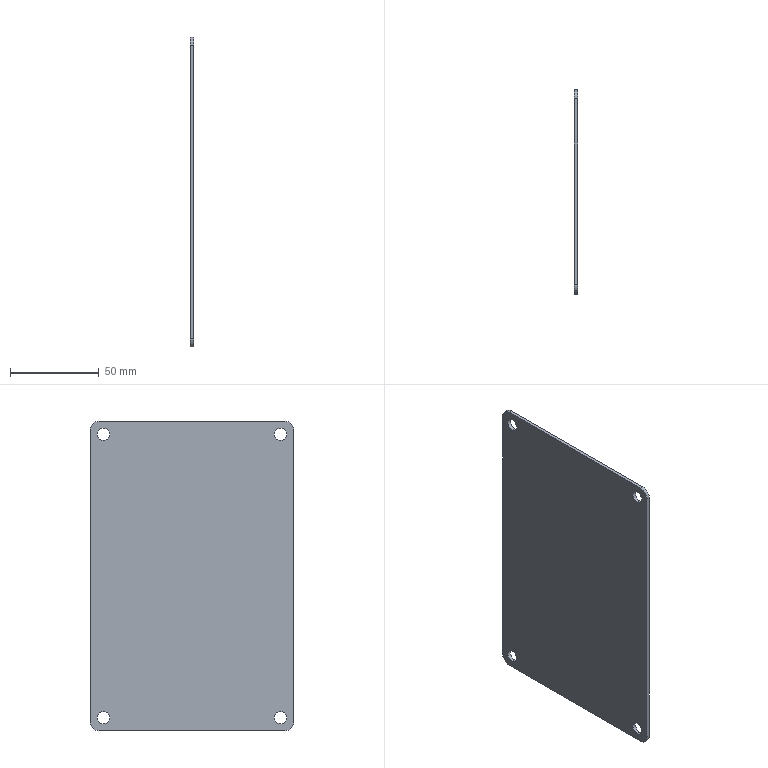Part | SolidWorks | 1 solid | 18 faces | box 2 x 115 x 175 mm | volume 39899 mm3 | cylinder 12 | plane 6 | commonest cylinder face diameters 7 x8 10 x4
STEP:
#1=CARTESIAN_POINT('',(-2.,-50.,76.5));
#2=VERTEX_POINT('',#1);
#3=CARTESIAN_POINT('',(-2.,-50.,83.5));
#4=VERTEX_POINT('',#3);
#5=CARTESIAN_POINT('',(-2.,-50.,80.));
#6=DIRECTION('',(-1.,0.,0.));
#7=DIRECTION('',(0.,0.,-1.));
#8=AXIS2_PLACEMENT_3D('',#5,#6,#7);
#9=CIRCLE('',#8,3.5);
#10=EDGE_CURVE('',#2,#4,#9,.T.);
#11=ORIENTED_EDGE('',*,*,#10,.T.);
#12=CARTESIAN_POINT('',(0.,-50.,83.5));
#13=VERTEX_POINT('',#12);
#14=CARTESIAN_POINT('',(-2.001,-50.,83.5));
#15=DIRECTION('',(1.,0.,0.));
#16=VECTOR('',#15,1000.);
#17=LINE('',#14,#16);
#18=EDGE_CURVE('',#4,#13,#17,.T.);
#19=ORIENTED_EDGE('',*,*,#18,.T.);
#20=CARTESIAN_POINT('',(0.,-50.,76.5));
#21=VERTEX_POINT('',#20);
#22=CARTESIAN_POINT('',(0.,-50.,80.));
#23=DIRECTION('',(1.,0.,0.));
#24=DIRECTION('',(0.,0.,-1.));
#25=AXIS2_PLACEMENT_3D('',#22,#23,#24);
#26=CIRCLE('',#25,3.5);
#27=EDGE_CURVE('',#13,#21,#26,.T.);
#28=ORIENTED_EDGE('',*,*,#27,.T.);
#29=CARTESIAN_POINT('',(-2.001,-50.,76.5));
#30=DIRECTION('',(1.,0.,0.));
#31=VECTOR('',#30,1000.);
#32=LINE('',#29,#31);
#33=EDGE_CURVE('',#2,#21,#32,.T.);
#34=ORIENTED_EDGE('',*,*,#33,.F.);
#35=EDGE_LOOP('',(#11,#19,#28,#34));
#36=FACE_OUTER_BOUND('',#35,.T.);
#37=CARTESIAN_POINT('',(-2.001,-50.,80.));
#38=DIRECTION('',(1.,0.,0.));
#39=DIRECTION('',(0.,0.,-1.));
#40=AXIS2_PLACEMENT_3D('',#37,#38,#39);
#41=CYLINDRICAL_SURFACE('',#40,3.5);
#42=ADVANCED_FACE('',(#36),#41,.F.);
#43=CARTESIAN_POINT('',(-2.,-50.,-83.5));
#44=VERTEX_POINT('',#43);
#45=CARTESIAN_POINT('',(-2.,-50.,-76.5));
#46=VERTEX_POINT('',#45);
#47=CARTESIAN_POINT('',(-2.,-50.,-80.));
#48=DIRECTION('',(-1.,0.,0.));
#49=DIRECTION('',(0.,0.,-1.));
#50=AXIS2_PLACEMENT_3D('',#47,#48,#49);
#51=CIRCLE('',#50,3.5);
#52=EDGE_CURVE('',#44,#46,#51,.T.);
#53=ORIENTED_EDGE('',*,*,#52,.T.);
#54=CARTESIAN_POINT('',(0.,-50.,-76.5));
#55=VERTEX_POINT('',#54);
#56=CARTESIAN_POINT('',(-2.001,-50.,-76.5));
#57=DIRECTION('',(1.,0.,0.));
#58=VECTOR('',#57,1000.);
#59=LINE('',#56,#58);
#60=EDGE_CURVE('',#46,#55,#59,.T.);
#61=ORIENTED_EDGE('',*,*,#60,.T.);
#62=CARTESIAN_POINT('',(0.,-50.,-83.5));
#63=VERTEX_POINT('',#62);
#64=CARTESIAN_POINT('',(0.,-50.,-80.));
#65=DIRECTION('',(1.,0.,0.));
#66=DIRECTION('',(0.,0.,-1.));
#67=AXIS2_PLACEMENT_3D('',#64,#65,#66);
#68=CIRCLE('',#67,3.5);
#69=EDGE_CURVE('',#55,#63,#68,.T.);
#70=ORIENTED_EDGE('',*,*,#69,.T.);
#71=CARTESIAN_POINT('',(-2.001,-50.,-83.5));
#72=DIRECTION('',(1.,0.,0.));
#73=VECTOR('',#72,1000.);
#74=LINE('',#71,#73);
#75=EDGE_CURVE('',#44,#63,#74,.T.);
#76=ORIENTED_EDGE('',*,*,#75,.F.);
#77=EDGE_LOOP('',(#53,#61,#70,#76));
#78=FACE_OUTER_BOUND('',#77,.T.);
#79=CARTESIAN_POINT('',(-2.001,-50.,-80.));
#80=DIRECTION('',(1.,0.,0.));
#81=DIRECTION('',(0.,0.,-1.));
#82=AXIS2_PLACEMENT_3D('',#79,#80,#81);
#83=CYLINDRICAL_SURFACE('',#82,3.5);
#84=ADVANCED_FACE('',(#78),#83,.F.);
#85=CARTESIAN_POINT('',(-2.,50.,-83.5));
#86=VERTEX_POINT('',#85);
#87=CARTESIAN_POINT('',(-2.,50.,-76.5));
#88=VERTEX_POINT('',#87);
#89=CARTESIAN_POINT('',(-2.,50.,-80.));
#90=DIRECTION('',(-1.,0.,0.));
#91=DIRECTION('',(0.,0.,-1.));
#92=AXIS2_PLACEMENT_3D('',#89,#90,#91);
#93=CIRCLE('',#92,3.5);
#94=EDGE_CURVE('',#86,#88,#93,.T.);
#95=ORIENTED_EDGE('',*,*,#94,.T.);
#96=CARTESIAN_POINT('',(0.,50.,-76.5));
#97=VERTEX_POINT('',#96);
#98=CARTESIAN_POINT('',(-2.001,50.,-76.5));
#99=DIRECTION('',(1.,0.,0.));
#100=VECTOR('',#99,1000.);
#101=LINE('',#98,#100);
#102=EDGE_CURVE('',#88,#97,#101,.T.);
#103=ORIENTED_EDGE('',*,*,#102,.T.);
#104=CARTESIAN_POINT('',(0.,50.,-83.5));
#105=VERTEX_POINT('',#104);
#106=CARTESIAN_POINT('',(0.,50.,-80.));
#107=DIRECTION('',(1.,0.,0.));
#108=DIRECTION('',(0.,0.,-1.));
#109=AXIS2_PLACEMENT_3D('',#106,#107,#108);
#110=CIRCLE('',#109,3.5);
#111=EDGE_CURVE('',#97,#105,#110,.T.);
#112=ORIENTED_EDGE('',*,*,#111,.T.);
#113=CARTESIAN_POINT('',(-2.001,50.,-83.5));
#114=DIRECTION('',(1.,0.,0.));
#115=VECTOR('',#114,1000.);
#116=LINE('',#113,#115);
#117=EDGE_CURVE('',#86,#105,#116,.T.);
#118=ORIENTED_EDGE('',*,*,#117,.F.);
#119=EDGE_LOOP('',(#95,#103,#112,#118));
#120=FACE_OUTER_BOUND('',#119,.T.);
#121=CARTESIAN_POINT('',(-2.001,50.,-80.));
#122=DIRECTION('',(1.,0.,0.));
#123=DIRECTION('',(0.,0.,-1.));
#124=AXIS2_PLACEMENT_3D('',#121,#122,#123);
#125=CYLINDRICAL_SURFACE('',#124,3.5);
#126=ADVANCED_FACE('',(#120),#125,.F.);
#127=CARTESIAN_POINT('',(-2.,50.,76.5));
#128=VERTEX_POINT('',#127);
#129=CARTESIAN_POINT('',(-2.,50.,83.5));
#130=VERTEX_POINT('',#129);
#131=CARTESIAN_POINT('',(-2.,50.,80.));
#132=DIRECTION('',(-1.,0.,0.));
#133=DIRECTION('',(0.,0.,-1.));
#134=AXIS2_PLACEMENT_3D('',#131,#132,#133);
#135=CIRCLE('',#134,3.5);
#136=EDGE_CURVE('',#128,#130,#135,.T.);
#137=ORIENTED_EDGE('',*,*,#136,.T.);
#138=CARTESIAN_POINT('',(0.,50.,83.5));
#139=VERTEX_POINT('',#138);
#140=CARTESIAN_POINT('',(-2.001,50.,83.5));
#141=DIRECTION('',(1.,0.,0.));
#142=VECTOR('',#141,1000.);
#143=LINE('',#140,#142);
#144=EDGE_CURVE('',#130,#139,#143,.T.);
#145=ORIENTED_EDGE('',*,*,#144,.T.);
#146=CARTESIAN_POINT('',(0.,50.,76.5));
#147=VERTEX_POINT('',#146);
#148=CARTESIAN_POINT('',(0.,50.,80.));
#149=DIRECTION('',(1.,0.,0.));
#150=DIRECTION('',(0.,0.,-1.));
#151=AXIS2_PLACEMENT_3D('',#148,#149,#150);
#152=CIRCLE('',#151,3.5);
#153=EDGE_CURVE('',#139,#147,#152,.T.);
#154=ORIENTED_EDGE('',*,*,#153,.T.);
#155=CARTESIAN_POINT('',(-2.001,50.,76.5));
#156=DIRECTION('',(1.,0.,0.));
#157=VECTOR('',#156,1000.);
#158=LINE('',#155,#157);
#159=EDGE_CURVE('',#128,#147,#158,.T.);
#160=ORIENTED_EDGE('',*,*,#159,.F.);
#161=EDGE_LOOP('',(#137,#145,#154,#160));
#162=FACE_OUTER_BOUND('',#161,.T.);
#163=CARTESIAN_POINT('',(-2.001,50.,80.));
#164=DIRECTION('',(1.,0.,0.));
#165=DIRECTION('',(0.,0.,-1.));
#166=AXIS2_PLACEMENT_3D('',#163,#164,#165);
#167=CYLINDRICAL_SURFACE('',#166,3.5);
#168=ADVANCED_FACE('',(#162),#167,.F.);
#169=CARTESIAN_POINT('',(-2.,52.5,87.5));
#170=VERTEX_POINT('',#169);
#171=CARTESIAN_POINT('',(-2.,-52.5,87.5));
#172=VERTEX_POINT('',#171);
#173=CARTESIAN_POINT('',(-2.,-57.5,87.5));
#174=DIRECTION('',(0.,-1.,0.));
#175=VECTOR('',#174,1000.);
#176=LINE('',#173,#175);
#177=EDGE_CURVE('',#170,#172,#176,.T.);
#178=ORIENTED_EDGE('',*,*,#177,.T.);
#179=CARTESIAN_POINT('',(0.,-52.5,87.5));
#180=VERTEX_POINT('',#179);
#181=CARTESIAN_POINT('',(-2.,-52.5,87.5));
#182=DIRECTION('',(1.,0.,0.));
#183=VECTOR('',#182,1000.);
#184=LINE('',#181,#183);
#185=EDGE_CURVE('',#172,#180,#184,.T.);
#186=ORIENTED_EDGE('',*,*,#185,.T.);
#187=CARTESIAN_POINT('',(0.,52.5,87.5));
#188=VERTEX_POINT('',#187);
#189=CARTESIAN_POINT('',(0.,-57.5,87.5));
#190=DIRECTION('',(0.,-1.,0.));
#191=VECTOR('',#190,1000.);
#192=LINE('',#189,#191);
#193=EDGE_CURVE('',#188,#180,#192,.T.);
#194=ORIENTED_EDGE('',*,*,#193,.F.);
#195=CARTESIAN_POINT('',(-2.,52.5,87.5));
#196=DIRECTION('',(-1.,0.,0.));
#197=VECTOR('',#196,1000.);
#198=LINE('',#195,#197);
#199=EDGE_CURVE('',#188,#170,#198,.T.);
#200=ORIENTED_EDGE('',*,*,#199,.T.);
#201=EDGE_LOOP('',(#178,#186,#194,#200));
#202=FACE_OUTER_BOUND('',#201,.T.);
#203=CARTESIAN_POINT('',(-2.,-57.5,87.5));
#204=DIRECTION('',(0.,0.,1.));
#205=DIRECTION('',(1.,0.,0.));
#206=AXIS2_PLACEMENT_3D('',#203,#204,#205);
#207=PLANE('',#206);
#208=ADVANCED_FACE('',(#202),#207,.T.);
#209=CARTESIAN_POINT('',(0.,57.5,-82.5));
#210=VERTEX_POINT('',#209);
#211=CARTESIAN_POINT('',(0.,57.5,82.5));
#212=VERTEX_POINT('',#211);
#213=CARTESIAN_POINT('',(0.,57.5,-87.5));
#214=DIRECTION('',(0.,0.,1.));
#215=VECTOR('',#214,1000.);
#216=LINE('',#213,#215);
#217=EDGE_CURVE('',#210,#212,#216,.T.);
#218=ORIENTED_EDGE('',*,*,#217,.F.);
#219=CARTESIAN_POINT('',(-2.,57.5,-82.5));
#220=VERTEX_POINT('',#219);
#221=CARTESIAN_POINT('',(-2.,57.5,-82.5));
#222=DIRECTION('',(-1.,0.,0.));
#223=VECTOR('',#222,1000.);
#224=LINE('',#221,#223);
#225=EDGE_CURVE('',#210,#220,#224,.T.);
#226=ORIENTED_EDGE('',*,*,#225,.T.);
#227=CARTESIAN_POINT('',(-2.,57.5,82.5));
#228=VERTEX_POINT('',#227);
#229=CARTESIAN_POINT('',(-2.,57.5,-87.5));
#230=DIRECTION('',(0.,0.,1.));
#231=VECTOR('',#230,1000.);
#232=LINE('',#229,#231);
#233=EDGE_CURVE('',#220,#228,#232,.T.);
#234=ORIENTED_EDGE('',*,*,#233,.T.);
#235=CARTESIAN_POINT('',(-2.,57.5,82.5));
#236=DIRECTION('',(1.,0.,0.));
#237=VECTOR('',#236,1000.);
#238=LINE('',#235,#237);
#239=EDGE_CURVE('',#228,#212,#238,.T.);
#240=ORIENTED_EDGE('',*,*,#239,.T.);
#241=EDGE_LOOP('',(#218,#226,#234,#240));
#242=FACE_OUTER_BOUND('',#241,.T.);
#243=CARTESIAN_POINT('',(-2.,57.5,-87.5));
#244=DIRECTION('',(0.,1.,0.));
#245=DIRECTION('',(0.,0.,1.));
#246=AXIS2_PLACEMENT_3D('',#243,#244,#245);
#247=PLANE('',#246);
#248=ADVANCED_FACE('',(#242),#247,.T.);
#249=CARTESIAN_POINT('',(0.,-52.5,-87.5));
#250=VERTEX_POINT('',#249);
#251=CARTESIAN_POINT('',(0.,52.5,-87.5));
#252=VERTEX_POINT('',#251);
#253=CARTESIAN_POINT('',(0.,-57.5,-87.5));
#254=DIRECTION('',(0.,1.,0.));
#255=VECTOR('',#254,1000.);
#256=LINE('',#253,#255);
#257=EDGE_CURVE('',#250,#252,#256,.T.);
#258=ORIENTED_EDGE('',*,*,#257,.F.);
#259=CARTESIAN_POINT('',(-2.,-52.5,-87.5));
#260=VERTEX_POINT('',#259);
#261=CARTESIAN_POINT('',(-2.,-52.5,-87.5));
#262=DIRECTION('',(-1.,0.,0.));
#263=VECTOR('',#262,1000.);
#264=LINE('',#261,#263);
#265=EDGE_CURVE('',#250,#260,#264,.T.);
#266=ORIENTED_EDGE('',*,*,#265,.T.);
#267=CARTESIAN_POINT('',(-2.,52.5,-87.5));
#268=VERTEX_POINT('',#267);
#269=CARTESIAN_POINT('',(-2.,-57.5,-87.5));
#270=DIRECTION('',(0.,1.,0.));
#271=VECTOR('',#270,1000.);
#272=LINE('',#269,#271);
#273=EDGE_CURVE('',#260,#268,#272,.T.);
#274=ORIENTED_EDGE('',*,*,#273,.T.);
#275=CARTESIAN_POINT('',(-2.,52.5,-87.5));
#276=DIRECTION('',(1.,0.,0.));
#277=VECTOR('',#276,1000.);
#278=LINE('',#275,#277);
#279=EDGE_CURVE('',#268,#252,#278,.T.);
#280=ORIENTED_EDGE('',*,*,#279,.T.);
#281=EDGE_LOOP('',(#258,#266,#274,#280));
#282=FACE_OUTER_BOUND('',#281,.T.);
#283=CARTESIAN_POINT('',(-2.,-57.5,-87.5));
#284=DIRECTION('',(0.,0.,-1.));
#285=DIRECTION('',(-1.,0.,0.));
#286=AXIS2_PLACEMENT_3D('',#283,#284,#285);
#287=PLANE('',#286);
#288=ADVANCED_FACE('',(#282),#287,.T.);
#289=CARTESIAN_POINT('',(0.,-57.5,82.5));
#290=VERTEX_POINT('',#289);
#291=CARTESIAN_POINT('',(0.,-57.5,-82.5));
#292=VERTEX_POINT('',#291);
#293=CARTESIAN_POINT('',(0.,-57.5,-87.5));
#294=DIRECTION('',(0.,0.,-1.));
#295=VECTOR('',#294,1000.);
#296=LINE('',#293,#295);
#297=EDGE_CURVE('',#290,#292,#296,.T.);
#298=ORIENTED_EDGE('',*,*,#297,.F.);
#299=CARTESIAN_POINT('',(-2.,-57.5,82.5));
#300=VERTEX_POINT('',#299);
#301=CARTESIAN_POINT('',(-2.,-57.5,82.5));
#302=DIRECTION('',(-1.,0.,0.));
#303=VECTOR('',#302,1000.);
#304=LINE('',#301,#303);
#305=EDGE_CURVE('',#290,#300,#304,.T.);
#306=ORIENTED_EDGE('',*,*,#305,.T.);
#307=CARTESIAN_POINT('',(-2.,-57.5,-82.5));
#308=VERTEX_POINT('',#307);
#309=CARTESIAN_POINT('',(-2.,-57.5,-87.5));
#310=DIRECTION('',(0.,0.,-1.));
#311=VECTOR('',#310,1000.);
#312=LINE('',#309,#311);
#313=EDGE_CURVE('',#300,#308,#312,.T.);
#314=ORIENTED_EDGE('',*,*,#313,.T.);
#315=CARTESIAN_POINT('',(-2.,-57.5,-82.5));
#316=DIRECTION('',(1.,0.,0.));
#317=VECTOR('',#316,1000.);
#318=LINE('',#315,#317);
#319=EDGE_CURVE('',#308,#292,#318,.T.);
#320=ORIENTED_EDGE('',*,*,#319,.T.);
#321=EDGE_LOOP('',(#298,#306,#314,#320));
#322=FACE_OUTER_BOUND('',#321,.T.);
#323=CARTESIAN_POINT('',(-2.,-57.5,-87.5));
#324=DIRECTION('',(0.,-1.,0.));
#325=DIRECTION('',(0.,0.,-1.));
#326=AXIS2_PLACEMENT_3D('',#323,#324,#325);
#327=PLANE('',#326);
#328=ADVANCED_FACE('',(#322),#327,.T.);
#329=ORIENTED_EDGE('',*,*,#10,.F.);
#330=CARTESIAN_POINT('',(-2.,-50.,80.));
#331=DIRECTION('',(-1.,0.,0.));
#332=DIRECTION('',(0.,0.,-1.));
#333=AXIS2_PLACEMENT_3D('',#330,#331,#332);
#334=CIRCLE('',#333,3.5);
#335=EDGE_CURVE('',#4,#2,#334,.T.);
#336=ORIENTED_EDGE('',*,*,#335,.F.);
#337=EDGE_LOOP('',(#329,#336));
#338=FACE_BOUND('',#337,.T.);
#339=ORIENTED_EDGE('',*,*,#52,.F.);
#340=CARTESIAN_POINT('',(-2.,-50.,-80.));
#341=DIRECTION('',(-1.,0.,0.));
#342=DIRECTION('',(0.,0.,-1.));
#343=AXIS2_PLACEMENT_3D('',#340,#341,#342);
#344=CIRCLE('',#343,3.5);
#345=EDGE_CURVE('',#46,#44,#344,.T.);
#346=ORIENTED_EDGE('',*,*,#345,.F.);
#347=EDGE_LOOP('',(#339,#346));
#348=FACE_BOUND('',#347,.T.);
#349=ORIENTED_EDGE('',*,*,#94,.F.);
#350=CARTESIAN_POINT('',(-2.,50.,-80.));
#351=DIRECTION('',(-1.,0.,0.));
#352=DIRECTION('',(0.,0.,-1.));
#353=AXIS2_PLACEMENT_3D('',#350,#351,#352);
#354=CIRCLE('',#353,3.5);
#355=EDGE_CURVE('',#88,#86,#354,.T.);
#356=ORIENTED_EDGE('',*,*,#355,.F.);
#357=EDGE_LOOP('',(#349,#356));
#358=FACE_BOUND('',#357,.T.);
#359=ORIENTED_EDGE('',*,*,#136,.F.);
#360=CARTESIAN_POINT('',(-2.,50.,80.));
#361=DIRECTION('',(-1.,0.,0.));
#362=DIRECTION('',(0.,0.,-1.));
#363=AXIS2_PLACEMENT_3D('',#360,#361,#362);
#364=CIRCLE('',#363,3.5);
#365=EDGE_CURVE('',#130,#128,#364,.T.);
#366=ORIENTED_EDGE('',*,*,#365,.F.);
#367=EDGE_LOOP('',(#359,#366));
#368=FACE_BOUND('',#367,.T.);
#369=ORIENTED_EDGE('',*,*,#313,.F.);
#370=CARTESIAN_POINT('',(-2.,-52.5,82.5));
#371=DIRECTION('',(-1.,0.,0.));
#372=DIRECTION('',(0.,0.,-1.));
#373=AXIS2_PLACEMENT_3D('',#370,#371,#372);
#374=CIRCLE('',#373,5.);
#375=EDGE_CURVE('',#300,#172,#374,.T.);
#376=ORIENTED_EDGE('',*,*,#375,.T.);
#377=ORIENTED_EDGE('',*,*,#177,.F.);
#378=CARTESIAN_POINT('',(-2.,52.5,82.5));
#379=DIRECTION('',(-1.,0.,0.));
#380=DIRECTION('',(0.,0.,-1.));
#381=AXIS2_PLACEMENT_3D('',#378,#379,#380);
#382=CIRCLE('',#381,5.);
#383=EDGE_CURVE('',#170,#228,#382,.T.);
#384=ORIENTED_EDGE('',*,*,#383,.T.);
#385=ORIENTED_EDGE('',*,*,#233,.F.);
#386=CARTESIAN_POINT('',(-2.,52.5,-82.5));
#387=DIRECTION('',(-1.,0.,0.));
#388=DIRECTION('',(0.,0.,-1.));
#389=AXIS2_PLACEMENT_3D('',#386,#387,#388);
#390=CIRCLE('',#389,5.);
#391=EDGE_CURVE('',#220,#268,#390,.T.);
#392=ORIENTED_EDGE('',*,*,#391,.T.);
#393=ORIENTED_EDGE('',*,*,#273,.F.);
#394=CARTESIAN_POINT('',(-2.,-52.5,-82.5));
#395=DIRECTION('',(-1.,0.,0.));
#396=DIRECTION('',(0.,0.,-1.));
#397=AXIS2_PLACEMENT_3D('',#394,#395,#396);
#398=CIRCLE('',#397,5.);
#399=EDGE_CURVE('',#260,#308,#398,.T.);
#400=ORIENTED_EDGE('',*,*,#399,.T.);
#401=EDGE_LOOP('',(#369,#376,#377,#384,#385,#392,#393,#400));
#402=FACE_OUTER_BOUND('',#401,.T.);
#403=CARTESIAN_POINT('',(-2.,0.,0.));
#404=DIRECTION('',(1.,0.,0.));
#405=DIRECTION('',(0.,0.,-1.));
#406=AXIS2_PLACEMENT_3D('',#403,#404,#405);
#407=PLANE('',#406);
#408=ADVANCED_FACE('',(#338,#348,#358,#368,#402),#407,.F.);
#409=CARTESIAN_POINT('',(0.,-50.,80.));
#410=DIRECTION('',(1.,0.,0.));
#411=DIRECTION('',(0.,0.,-1.));
#412=AXIS2_PLACEMENT_3D('',#409,#410,#411);
#413=CIRCLE('',#412,3.5);
#414=EDGE_CURVE('',#21,#13,#413,.T.);
#415=ORIENTED_EDGE('',*,*,#414,.F.);
#416=ORIENTED_EDGE('',*,*,#27,.F.);
#417=EDGE_LOOP('',(#415,#416));
#418=FACE_BOUND('',#417,.T.);
#419=CARTESIAN_POINT('',(0.,-50.,-80.));
#420=DIRECTION('',(1.,0.,0.));
#421=DIRECTION('',(0.,0.,-1.));
#422=AXIS2_PLACEMENT_3D('',#419,#420,#421);
#423=CIRCLE('',#422,3.5);
#424=EDGE_CURVE('',#63,#55,#423,.T.);
#425=ORIENTED_EDGE('',*,*,#424,.F.);
#426=ORIENTED_EDGE('',*,*,#69,.F.);
#427=EDGE_LOOP('',(#425,#426));
#428=FACE_BOUND('',#427,.T.);
#429=CARTESIAN_POINT('',(0.,50.,-80.));
#430=DIRECTION('',(1.,0.,0.));
#431=DIRECTION('',(0.,0.,-1.));
#432=AXIS2_PLACEMENT_3D('',#429,#430,#431);
#433=CIRCLE('',#432,3.5);
#434=EDGE_CURVE('',#105,#97,#433,.T.);
#435=ORIENTED_EDGE('',*,*,#434,.F.);
#436=ORIENTED_EDGE('',*,*,#111,.F.);
#437=EDGE_LOOP('',(#435,#436));
#438=FACE_BOUND('',#437,.T.);
#439=CARTESIAN_POINT('',(0.,50.,80.));
#440=DIRECTION('',(1.,0.,0.));
#441=DIRECTION('',(0.,0.,-1.));
#442=AXIS2_PLACEMENT_3D('',#439,#440,#441);
#443=CIRCLE('',#442,3.5);
#444=EDGE_CURVE('',#147,#139,#443,.T.);
#445=ORIENTED_EDGE('',*,*,#444,.F.);
#446=ORIENTED_EDGE('',*,*,#153,.F.);
#447=EDGE_LOOP('',(#445,#446));
#448=FACE_BOUND('',#447,.T.);
#449=ORIENTED_EDGE('',*,*,#193,.T.);
#450=CARTESIAN_POINT('',(0.,-52.5,82.5));
#451=DIRECTION('',(1.,0.,0.));
#452=DIRECTION('',(0.,0.,-1.));
#453=AXIS2_PLACEMENT_3D('',#450,#451,#452);
#454=CIRCLE('',#453,5.);
#455=EDGE_CURVE('',#180,#290,#454,.T.);
#456=ORIENTED_EDGE('',*,*,#455,.T.);
#457=ORIENTED_EDGE('',*,*,#297,.T.);
#458=CARTESIAN_POINT('',(0.,-52.5,-82.5));
#459=DIRECTION('',(1.,0.,0.));
#460=DIRECTION('',(0.,0.,-1.));
#461=AXIS2_PLACEMENT_3D('',#458,#459,#460);
#462=CIRCLE('',#461,5.);
#463=EDGE_CURVE('',#292,#250,#462,.T.);
#464=ORIENTED_EDGE('',*,*,#463,.T.);
#465=ORIENTED_EDGE('',*,*,#257,.T.);
#466=CARTESIAN_POINT('',(0.,52.5,-82.5));
#467=DIRECTION('',(1.,0.,0.));
#468=DIRECTION('',(0.,0.,-1.));
#469=AXIS2_PLACEMENT_3D('',#466,#467,#468);
#470=CIRCLE('',#469,5.);
#471=EDGE_CURVE('',#252,#210,#470,.T.);
#472=ORIENTED_EDGE('',*,*,#471,.T.);
#473=ORIENTED_EDGE('',*,*,#217,.T.);
#474=CARTESIAN_POINT('',(0.,52.5,82.5));
#475=DIRECTION('',(1.,0.,0.));
#476=DIRECTION('',(0.,0.,-1.));
#477=AXIS2_PLACEMENT_3D('',#474,#475,#476);
#478=CIRCLE('',#477,5.);
#479=EDGE_CURVE('',#212,#188,#478,.T.);
#480=ORIENTED_EDGE('',*,*,#479,.T.);
#481=EDGE_LOOP('',(#449,#456,#457,#464,#465,#472,#473,#480));
#482=FACE_OUTER_BOUND('',#481,.T.);
#483=CARTESIAN_POINT('',(0.,0.,0.));
#484=DIRECTION('',(1.,0.,0.));
#485=DIRECTION('',(0.,0.,-1.));
#486=AXIS2_PLACEMENT_3D('',#483,#484,#485);
#487=PLANE('',#486);
#488=ADVANCED_FACE('',(#418,#428,#438,#448,#482),#487,.T.);
#489=ORIENTED_EDGE('',*,*,#144,.F.);
#490=ORIENTED_EDGE('',*,*,#365,.T.);
#491=ORIENTED_EDGE('',*,*,#159,.T.);
#492=ORIENTED_EDGE('',*,*,#444,.T.);
#493=EDGE_LOOP('',(#489,#490,#491,#492));
#494=FACE_OUTER_BOUND('',#493,.T.);
#495=CARTESIAN_POINT('',(-2.001,50.,80.));
#496=DIRECTION('',(1.,0.,0.));
#497=DIRECTION('',(0.,0.,-1.));
#498=AXIS2_PLACEMENT_3D('',#495,#496,#497);
#499=CYLINDRICAL_SURFACE('',#498,3.5);
#500=ADVANCED_FACE('',(#494),#499,.F.);
#501=ORIENTED_EDGE('',*,*,#102,.F.);
#502=ORIENTED_EDGE('',*,*,#355,.T.);
#503=ORIENTED_EDGE('',*,*,#117,.T.);
#504=ORIENTED_EDGE('',*,*,#434,.T.);
#505=EDGE_LOOP('',(#501,#502,#503,#504));
#506=FACE_OUTER_BOUND('',#505,.T.);
#507=CARTESIAN_POINT('',(-2.001,50.,-80.));
#508=DIRECTION('',(1.,0.,0.));
#509=DIRECTION('',(0.,0.,-1.));
#510=AXIS2_PLACEMENT_3D('',#507,#508,#509);
#511=CYLINDRICAL_SURFACE('',#510,3.5);
#512=ADVANCED_FACE('',(#506),#511,.F.);
#513=ORIENTED_EDGE('',*,*,#60,.F.);
#514=ORIENTED_EDGE('',*,*,#345,.T.);
#515=ORIENTED_EDGE('',*,*,#75,.T.);
#516=ORIENTED_EDGE('',*,*,#424,.T.);
#517=EDGE_LOOP('',(#513,#514,#515,#516));
#518=FACE_OUTER_BOUND('',#517,.T.);
#519=CARTESIAN_POINT('',(-2.001,-50.,-80.));
#520=DIRECTION('',(1.,0.,0.));
#521=DIRECTION('',(0.,0.,-1.));
#522=AXIS2_PLACEMENT_3D('',#519,#520,#521);
#523=CYLINDRICAL_SURFACE('',#522,3.5);
#524=ADVANCED_FACE('',(#518),#523,.F.);
#525=ORIENTED_EDGE('',*,*,#18,.F.);
#526=ORIENTED_EDGE('',*,*,#335,.T.);
#527=ORIENTED_EDGE('',*,*,#33,.T.);
#528=ORIENTED_EDGE('',*,*,#414,.T.);
#529=EDGE_LOOP('',(#525,#526,#527,#528));
#530=FACE_OUTER_BOUND('',#529,.T.);
#531=CARTESIAN_POINT('',(-2.001,-50.,80.));
#532=DIRECTION('',(1.,0.,0.));
#533=DIRECTION('',(0.,0.,-1.));
#534=AXIS2_PLACEMENT_3D('',#531,#532,#533);
#535=CYLINDRICAL_SURFACE('',#534,3.5);
#536=ADVANCED_FACE('',(#530),#535,.F.);
#537=ORIENTED_EDGE('',*,*,#375,.F.);
#538=ORIENTED_EDGE('',*,*,#305,.F.);
#539=ORIENTED_EDGE('',*,*,#455,.F.);
#540=ORIENTED_EDGE('',*,*,#185,.F.);
#541=EDGE_LOOP('',(#537,#538,#539,#540));
#542=FACE_OUTER_BOUND('',#541,.T.);
#543=CARTESIAN_POINT('',(-2.,-52.5,82.5));
#544=DIRECTION('',(1.,0.,0.));
#545=DIRECTION('',(0.,0.,-1.));
#546=AXIS2_PLACEMENT_3D('',#543,#544,#545);
#547=CYLINDRICAL_SURFACE('',#546,5.);
#548=ADVANCED_FACE('',(#542),#547,.T.);
#549=ORIENTED_EDGE('',*,*,#399,.F.);
#550=ORIENTED_EDGE('',*,*,#265,.F.);
#551=ORIENTED_EDGE('',*,*,#463,.F.);
#552=ORIENTED_EDGE('',*,*,#319,.F.);
#553=EDGE_LOOP('',(#549,#550,#551,#552));
#554=FACE_OUTER_BOUND('',#553,.T.);
#555=CARTESIAN_POINT('',(-2.,-52.5,-82.5));
#556=DIRECTION('',(1.,0.,0.));
#557=DIRECTION('',(0.,0.,-1.));
#558=AXIS2_PLACEMENT_3D('',#555,#556,#557);
#559=CYLINDRICAL_SURFACE('',#558,5.);
#560=ADVANCED_FACE('',(#554),#559,.T.);
#561=ORIENTED_EDGE('',*,*,#391,.F.);
#562=ORIENTED_EDGE('',*,*,#225,.F.);
#563=ORIENTED_EDGE('',*,*,#471,.F.);
#564=ORIENTED_EDGE('',*,*,#279,.F.);
#565=EDGE_LOOP('',(#561,#562,#563,#564));
#566=FACE_OUTER_BOUND('',#565,.T.);
#567=CARTESIAN_POINT('',(-2.,52.5,-82.5));
#568=DIRECTION('',(1.,0.,0.));
#569=DIRECTION('',(0.,0.,-1.));
#570=AXIS2_PLACEMENT_3D('',#567,#568,#569);
#571=CYLINDRICAL_SURFACE('',#570,5.);
#572=ADVANCED_FACE('',(#566),#571,.T.);
#573=ORIENTED_EDGE('',*,*,#383,.F.);
#574=ORIENTED_EDGE('',*,*,#199,.F.);
#575=ORIENTED_EDGE('',*,*,#479,.F.);
#576=ORIENTED_EDGE('',*,*,#239,.F.);
#577=EDGE_LOOP('',(#573,#574,#575,#576));
#578=FACE_OUTER_BOUND('',#577,.T.);
#579=CARTESIAN_POINT('',(-2.,52.5,82.5));
#580=DIRECTION('',(1.,0.,0.));
#581=DIRECTION('',(0.,0.,-1.));
#582=AXIS2_PLACEMENT_3D('',#579,#580,#581);
#583=CYLINDRICAL_SURFACE('',#582,5.);
#584=ADVANCED_FACE('',(#578),#583,.T.);
#585=CLOSED_SHELL('',(#42,#84,#126,#168,#208,#248,#288,#328,#408,#488,#500,#512,#524,#536,#548,#560,#572,#584));
#586=MANIFOLD_SOLID_BREP('',#585);
#587=CARTESIAN_POINT('',(0.,0.,0.));
#588=DIRECTION('',(0.,0.,1.));
#589=DIRECTION('',(1.,0.,0.));
#590=AXIS2_PLACEMENT_3D('',#587,#588,#589);
#591=(LENGTH_UNIT()NAMED_UNIT(*)SI_UNIT(.MILLI.,.METRE.));
#592=UNCERTAINTY_MEASURE_WITH_UNIT(LENGTH_MEASURE(0.00001),#591,'','');
#593=(NAMED_UNIT(*)PLANE_ANGLE_UNIT()SI_UNIT($,.RADIAN.));
#594=(NAMED_UNIT(*)SI_UNIT($,.STERADIAN.)SOLID_ANGLE_UNIT());
#595=(GEOMETRIC_REPRESENTATION_CONTEXT(3)GLOBAL_UNCERTAINTY_ASSIGNED_CONTEXT((#592))GLOBAL_UNIT_ASSIGNED_CONTEXT((#591,#593,#594))REPRESENTATION_CONTEXT('',''));
#596=ADVANCED_BREP_SHAPE_REPRESENTATION('',(#586,#590),#595);